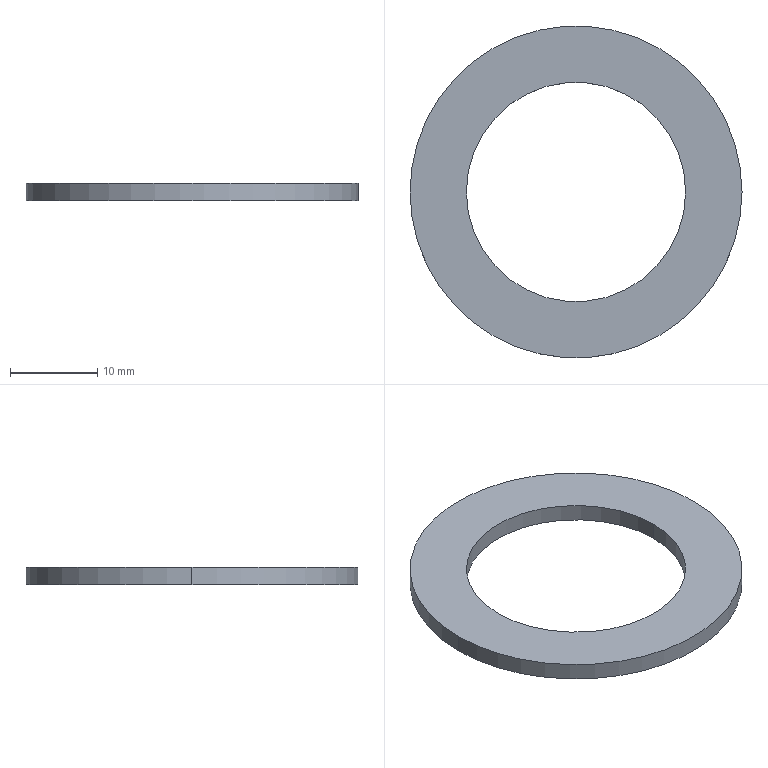Part | NX | 1 solid | 6 faces | box 38 x 38 x 2 mm | volume 1279 mm3 | cylinder 4 | plane 2 | commonest cylinder face diameters 25.1 x2 38 x2
STEP:
#1=CARTESIAN_POINT('',(-19.,0.,0.));
#2=VERTEX_POINT('',#1);
#3=CARTESIAN_POINT('',(19.,0.,0.));
#4=VERTEX_POINT('',#3);
#5=CARTESIAN_POINT('',(0.,0.,0.));
#6=DIRECTION('',(0.,0.,1.));
#7=DIRECTION('',(1.,0.,0.));
#8=AXIS2_PLACEMENT_3D('',#5,#6,#7);
#9=CIRCLE('',#8,19.);
#10=EDGE_CURVE('',#2,#4,#9,.T.);
#11=ORIENTED_EDGE('',*,*,#10,.F.);
#12=CARTESIAN_POINT('',(0.,0.,0.));
#13=DIRECTION('',(0.,0.,1.));
#14=DIRECTION('',(1.,0.,0.));
#15=AXIS2_PLACEMENT_3D('',#12,#13,#14);
#16=CIRCLE('',#15,19.);
#17=EDGE_CURVE('',#4,#2,#16,.T.);
#18=ORIENTED_EDGE('',*,*,#17,.F.);
#19=EDGE_LOOP('',(#11,#18));
#20=FACE_BOUND('',#19,.T.);
#21=CARTESIAN_POINT('',(-12.55,0.,0.));
#22=VERTEX_POINT('',#21);
#23=CARTESIAN_POINT('',(12.55,0.,0.));
#24=VERTEX_POINT('',#23);
#25=CARTESIAN_POINT('',(0.,0.,0.));
#26=DIRECTION('',(0.,0.,1.));
#27=DIRECTION('',(1.,0.,0.));
#28=AXIS2_PLACEMENT_3D('',#25,#26,#27);
#29=CIRCLE('',#28,12.55);
#30=EDGE_CURVE('',#22,#24,#29,.T.);
#31=ORIENTED_EDGE('',*,*,#30,.T.);
#32=CARTESIAN_POINT('',(0.,0.,0.));
#33=DIRECTION('',(0.,0.,1.));
#34=DIRECTION('',(1.,0.,0.));
#35=AXIS2_PLACEMENT_3D('',#32,#33,#34);
#36=CIRCLE('',#35,12.55);
#37=EDGE_CURVE('',#24,#22,#36,.T.);
#38=ORIENTED_EDGE('',*,*,#37,.T.);
#39=EDGE_LOOP('',(#31,#38));
#40=FACE_BOUND('',#39,.T.);
#41=CARTESIAN_POINT('',(0.,0.,0.));
#42=DIRECTION('',(0.,0.,1.));
#43=DIRECTION('',(1.,0.,0.));
#44=AXIS2_PLACEMENT_3D('',#41,#42,#43);
#45=PLANE('',#44);
#46=ADVANCED_FACE('',(#20,#40),#45,.F.);
#47=CARTESIAN_POINT('',(-19.,0.,2.));
#48=VERTEX_POINT('',#47);
#49=CARTESIAN_POINT('',(19.,0.,2.));
#50=VERTEX_POINT('',#49);
#51=CARTESIAN_POINT('',(0.,0.,2.));
#52=DIRECTION('',(0.,0.,1.));
#53=DIRECTION('',(1.,0.,0.));
#54=AXIS2_PLACEMENT_3D('',#51,#52,#53);
#55=CIRCLE('',#54,19.);
#56=EDGE_CURVE('',#48,#50,#55,.T.);
#57=ORIENTED_EDGE('',*,*,#56,.F.);
#58=CARTESIAN_POINT('',(-19.,0.,0.));
#59=DIRECTION('',(0.,0.,1.));
#60=VECTOR('',#59,1000.);
#61=LINE('',#58,#60);
#62=EDGE_CURVE('',#2,#48,#61,.T.);
#63=ORIENTED_EDGE('',*,*,#62,.F.);
#64=ORIENTED_EDGE('',*,*,#10,.T.);
#65=CARTESIAN_POINT('',(19.,0.,0.));
#66=DIRECTION('',(0.,0.,1.));
#67=VECTOR('',#66,1000.);
#68=LINE('',#65,#67);
#69=EDGE_CURVE('',#4,#50,#68,.T.);
#70=ORIENTED_EDGE('',*,*,#69,.T.);
#71=EDGE_LOOP('',(#57,#63,#64,#70));
#72=FACE_BOUND('',#71,.T.);
#73=CARTESIAN_POINT('',(0.,0.,0.));
#74=DIRECTION('',(0.,0.,1.));
#75=DIRECTION('',(1.,0.,0.));
#76=AXIS2_PLACEMENT_3D('',#73,#74,#75);
#77=CYLINDRICAL_SURFACE('',#76,19.);
#78=ADVANCED_FACE('',(#72),#77,.T.);
#79=ORIENTED_EDGE('',*,*,#30,.F.);
#80=CARTESIAN_POINT('',(-12.55,0.,2.));
#81=VERTEX_POINT('',#80);
#82=CARTESIAN_POINT('',(-12.55,0.,0.));
#83=DIRECTION('',(0.,0.,1.));
#84=VECTOR('',#83,1000.);
#85=LINE('',#82,#84);
#86=EDGE_CURVE('',#81,#22,#85,.F.);
#87=ORIENTED_EDGE('',*,*,#86,.F.);
#88=CARTESIAN_POINT('',(12.55,0.,2.));
#89=VERTEX_POINT('',#88);
#90=CARTESIAN_POINT('',(0.,0.,2.));
#91=DIRECTION('',(0.,0.,1.));
#92=DIRECTION('',(1.,0.,0.));
#93=AXIS2_PLACEMENT_3D('',#90,#91,#92);
#94=CIRCLE('',#93,12.55);
#95=EDGE_CURVE('',#81,#89,#94,.T.);
#96=ORIENTED_EDGE('',*,*,#95,.T.);
#97=CARTESIAN_POINT('',(12.55,0.,0.));
#98=DIRECTION('',(0.,0.,1.));
#99=VECTOR('',#98,1000.);
#100=LINE('',#97,#99);
#101=EDGE_CURVE('',#89,#24,#100,.F.);
#102=ORIENTED_EDGE('',*,*,#101,.T.);
#103=EDGE_LOOP('',(#79,#87,#96,#102));
#104=FACE_BOUND('',#103,.T.);
#105=CARTESIAN_POINT('',(0.,0.,0.));
#106=DIRECTION('',(0.,0.,1.));
#107=DIRECTION('',(1.,0.,0.));
#108=AXIS2_PLACEMENT_3D('',#105,#106,#107);
#109=CYLINDRICAL_SURFACE('',#108,12.55);
#110=ADVANCED_FACE('',(#104),#109,.F.);
#111=ORIENTED_EDGE('',*,*,#56,.T.);
#112=CARTESIAN_POINT('',(0.,0.,2.));
#113=DIRECTION('',(0.,0.,1.));
#114=DIRECTION('',(1.,0.,0.));
#115=AXIS2_PLACEMENT_3D('',#112,#113,#114);
#116=CIRCLE('',#115,19.);
#117=EDGE_CURVE('',#50,#48,#116,.T.);
#118=ORIENTED_EDGE('',*,*,#117,.T.);
#119=EDGE_LOOP('',(#111,#118));
#120=FACE_BOUND('',#119,.T.);
#121=CARTESIAN_POINT('',(0.,0.,2.));
#122=DIRECTION('',(0.,0.,1.));
#123=DIRECTION('',(1.,0.,0.));
#124=AXIS2_PLACEMENT_3D('',#121,#122,#123);
#125=CIRCLE('',#124,12.55);
#126=EDGE_CURVE('',#89,#81,#125,.T.);
#127=ORIENTED_EDGE('',*,*,#126,.F.);
#128=ORIENTED_EDGE('',*,*,#95,.F.);
#129=EDGE_LOOP('',(#127,#128));
#130=FACE_BOUND('',#129,.T.);
#131=CARTESIAN_POINT('',(0.,0.,2.));
#132=DIRECTION('',(0.,0.,1.));
#133=DIRECTION('',(1.,0.,0.));
#134=AXIS2_PLACEMENT_3D('',#131,#132,#133);
#135=PLANE('',#134);
#136=ADVANCED_FACE('',(#120,#130),#135,.T.);
#137=ORIENTED_EDGE('',*,*,#69,.F.);
#138=ORIENTED_EDGE('',*,*,#17,.T.);
#139=ORIENTED_EDGE('',*,*,#62,.T.);
#140=ORIENTED_EDGE('',*,*,#117,.F.);
#141=EDGE_LOOP('',(#137,#138,#139,#140));
#142=FACE_BOUND('',#141,.T.);
#143=CARTESIAN_POINT('',(0.,0.,0.));
#144=DIRECTION('',(0.,0.,1.));
#145=DIRECTION('',(1.,0.,0.));
#146=AXIS2_PLACEMENT_3D('',#143,#144,#145);
#147=CYLINDRICAL_SURFACE('',#146,19.);
#148=ADVANCED_FACE('',(#142),#147,.T.);
#149=ORIENTED_EDGE('',*,*,#126,.T.);
#150=ORIENTED_EDGE('',*,*,#86,.T.);
#151=ORIENTED_EDGE('',*,*,#37,.F.);
#152=ORIENTED_EDGE('',*,*,#101,.F.);
#153=EDGE_LOOP('',(#149,#150,#151,#152));
#154=FACE_BOUND('',#153,.T.);
#155=CARTESIAN_POINT('',(0.,0.,0.));
#156=DIRECTION('',(0.,0.,1.));
#157=DIRECTION('',(1.,0.,0.));
#158=AXIS2_PLACEMENT_3D('',#155,#156,#157);
#159=CYLINDRICAL_SURFACE('',#158,12.55);
#160=ADVANCED_FACE('',(#154),#159,.F.);
#161=CLOSED_SHELL('',(#46,#78,#110,#136,#148,#160));
#162=MANIFOLD_SOLID_BREP('',#161);
#163=(LENGTH_UNIT()NAMED_UNIT(*)SI_UNIT(.MILLI.,.METRE.));
#164=UNCERTAINTY_MEASURE_WITH_UNIT(LENGTH_MEASURE(0.00001),#163,'','');
#165=(NAMED_UNIT(*)PLANE_ANGLE_UNIT()SI_UNIT($,.RADIAN.));
#166=(NAMED_UNIT(*)SI_UNIT($,.STERADIAN.)SOLID_ANGLE_UNIT());
#167=(GEOMETRIC_REPRESENTATION_CONTEXT(3)GLOBAL_UNCERTAINTY_ASSIGNED_CONTEXT((#164))GLOBAL_UNIT_ASSIGNED_CONTEXT((#163,#165,#166))REPRESENTATION_CONTEXT('',''));
#168=ADVANCED_BREP_SHAPE_REPRESENTATION('',(#162),#167);